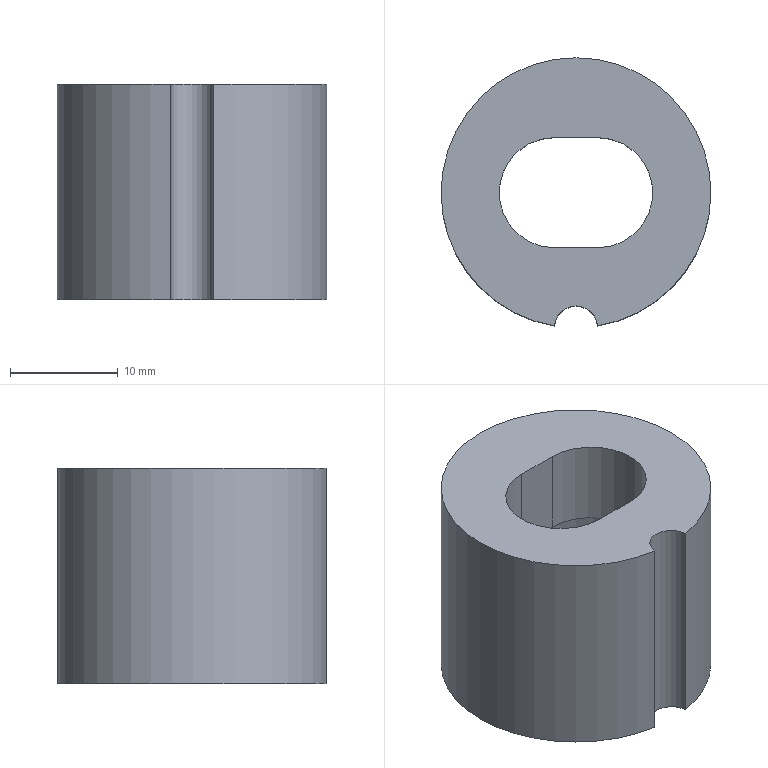Part | NX | features solid 2 | 1 solid | 10 faces | box 25 x 24.84 x 20 mm | volume 6116 mm3 | plane 5 | cylinder 5 | commonest cylinder face diameters 10.22 x2 4 x1 16.6 x1 25 x1
STEP:
#1=CARTESIAN_POINT('',(299.802,7.404,-5.344));
#2=VERTEX_POINT('',#1);
#3=CARTESIAN_POINT('',(303.789,7.404,-5.344));
#4=VERTEX_POINT('',#3);
#5=CARTESIAN_POINT('',(301.795,7.244,-5.344));
#6=DIRECTION('',(0.,0.,-1.));
#7=DIRECTION('',(0.,1.,0.));
#8=AXIS2_PLACEMENT_3D('',#5,#6,#7);
#9=CIRCLE('',#8,2.);
#10=EDGE_CURVE('',#2,#4,#9,.T.);
#11=ORIENTED_EDGE('',*,*,#10,.T.);
#12=CARTESIAN_POINT('',(301.795,19.744,-5.344));
#13=DIRECTION('',(0.,0.,-1.));
#14=DIRECTION('',(0.,1.,0.));
#15=AXIS2_PLACEMENT_3D('',#12,#13,#14);
#16=CIRCLE('',#15,12.5);
#17=EDGE_CURVE('',#2,#4,#16,.T.);
#18=ORIENTED_EDGE('',*,*,#17,.F.);
#19=EDGE_LOOP('',(#11,#18));
#20=FACE_BOUND('',#19,.T.);
#21=CARTESIAN_POINT('',(303.795,24.854,-5.344));
#22=VERTEX_POINT('',#21);
#23=CARTESIAN_POINT('',(303.795,14.634,-5.344));
#24=VERTEX_POINT('',#23);
#25=CARTESIAN_POINT('',(303.795,19.744,-5.344));
#26=DIRECTION('',(0.,0.,-1.));
#27=DIRECTION('',(0.,1.,0.));
#28=AXIS2_PLACEMENT_3D('',#25,#26,#27);
#29=CIRCLE('',#28,5.11);
#30=EDGE_CURVE('',#22,#24,#29,.T.);
#31=ORIENTED_EDGE('',*,*,#30,.T.);
#32=CARTESIAN_POINT('',(299.795,14.634,-5.344));
#33=VERTEX_POINT('',#32);
#34=CARTESIAN_POINT('',(301.795,14.634,-5.344));
#35=DIRECTION('',(-1.,0.,0.));
#36=VECTOR('',#35,1000.);
#37=LINE('',#34,#36);
#38=EDGE_CURVE('',#24,#33,#37,.T.);
#39=ORIENTED_EDGE('',*,*,#38,.T.);
#40=CARTESIAN_POINT('',(299.795,24.854,-5.344));
#41=VERTEX_POINT('',#40);
#42=CARTESIAN_POINT('',(299.795,19.744,-5.344));
#43=DIRECTION('',(0.,0.,-1.));
#44=DIRECTION('',(0.,1.,0.));
#45=AXIS2_PLACEMENT_3D('',#42,#43,#44);
#46=CIRCLE('',#45,5.11);
#47=EDGE_CURVE('',#33,#41,#46,.T.);
#48=ORIENTED_EDGE('',*,*,#47,.T.);
#49=CARTESIAN_POINT('',(301.795,24.854,-5.344));
#50=DIRECTION('',(1.,0.,0.));
#51=VECTOR('',#50,1000.);
#52=LINE('',#49,#51);
#53=EDGE_CURVE('',#41,#22,#52,.T.);
#54=ORIENTED_EDGE('',*,*,#53,.T.);
#55=EDGE_LOOP('',(#31,#39,#48,#54));
#56=FACE_BOUND('',#55,.T.);
#57=CARTESIAN_POINT('',(301.795,19.744,-5.344));
#58=DIRECTION('',(0.,0.,1.));
#59=DIRECTION('',(0.,-1.,0.));
#60=AXIS2_PLACEMENT_3D('',#57,#58,#59);
#61=PLANE('',#60);
#62=ADVANCED_FACE('',(#20,#56),#61,.T.);
#63=CARTESIAN_POINT('',(303.789,7.404,-25.344));
#64=VERTEX_POINT('',#63);
#65=CARTESIAN_POINT('',(299.802,7.404,-25.344));
#66=VERTEX_POINT('',#65);
#67=CARTESIAN_POINT('',(301.795,7.244,-25.344));
#68=DIRECTION('',(0.,0.,1.));
#69=DIRECTION('',(0.,-1.,0.));
#70=AXIS2_PLACEMENT_3D('',#67,#68,#69);
#71=CIRCLE('',#70,2.);
#72=EDGE_CURVE('',#64,#66,#71,.T.);
#73=ORIENTED_EDGE('',*,*,#72,.T.);
#74=CARTESIAN_POINT('',(301.795,19.744,-25.344));
#75=DIRECTION('',(0.,0.,1.));
#76=DIRECTION('',(0.,-1.,0.));
#77=AXIS2_PLACEMENT_3D('',#74,#75,#76);
#78=CIRCLE('',#77,12.5);
#79=EDGE_CURVE('',#64,#66,#78,.T.);
#80=ORIENTED_EDGE('',*,*,#79,.F.);
#81=EDGE_LOOP('',(#73,#80));
#82=FACE_BOUND('',#81,.T.);
#83=CARTESIAN_POINT('',(301.795,11.444,-25.344));
#84=VERTEX_POINT('',#83);
#85=CARTESIAN_POINT('',(301.795,19.744,-25.344));
#86=DIRECTION('',(0.,0.,1.));
#87=DIRECTION('',(0.,-1.,0.));
#88=AXIS2_PLACEMENT_3D('',#85,#86,#87);
#89=CIRCLE('',#88,8.3);
#90=EDGE_CURVE('',#84,#84,#89,.T.);
#91=ORIENTED_EDGE('',*,*,#90,.T.);
#92=EDGE_LOOP('',(#91));
#93=FACE_BOUND('',#92,.T.);
#94=CARTESIAN_POINT('',(301.795,19.744,-25.344));
#95=DIRECTION('',(0.,0.,-1.));
#96=DIRECTION('',(0.,1.,0.));
#97=AXIS2_PLACEMENT_3D('',#94,#95,#96);
#98=PLANE('',#97);
#99=ADVANCED_FACE('',(#82,#93),#98,.T.);
#100=CARTESIAN_POINT('',(303.789,7.404,-15.344));
#101=DIRECTION('',(0.,0.,1.));
#102=VECTOR('',#101,1000.);
#103=LINE('',#100,#102);
#104=EDGE_CURVE('',#64,#4,#103,.T.);
#105=ORIENTED_EDGE('',*,*,#104,.F.);
#106=ORIENTED_EDGE('',*,*,#79,.T.);
#107=CARTESIAN_POINT('',(299.802,7.404,-15.344));
#108=DIRECTION('',(0.,0.,1.));
#109=VECTOR('',#108,1000.);
#110=LINE('',#107,#109);
#111=EDGE_CURVE('',#2,#66,#110,.F.);
#112=ORIENTED_EDGE('',*,*,#111,.F.);
#113=ORIENTED_EDGE('',*,*,#17,.T.);
#114=EDGE_LOOP('',(#105,#106,#112,#113));
#115=FACE_BOUND('',#114,.T.);
#116=CARTESIAN_POINT('',(301.795,19.744,-25.344));
#117=DIRECTION('',(0.,0.,1.));
#118=DIRECTION('',(0.,-1.,0.));
#119=AXIS2_PLACEMENT_3D('',#116,#117,#118);
#120=CYLINDRICAL_SURFACE('',#119,12.5);
#121=ADVANCED_FACE('',(#115),#120,.T.);
#122=CARTESIAN_POINT('',(299.795,14.634,-13.344));
#123=VERTEX_POINT('',#122);
#124=CARTESIAN_POINT('',(303.795,14.634,-13.344));
#125=VERTEX_POINT('',#124);
#126=CARTESIAN_POINT('',(301.795,14.634,-13.344));
#127=DIRECTION('',(1.,0.,0.));
#128=VECTOR('',#127,1000.);
#129=LINE('',#126,#128);
#130=EDGE_CURVE('',#123,#125,#129,.T.);
#131=ORIENTED_EDGE('',*,*,#130,.T.);
#132=CARTESIAN_POINT('',(303.795,24.854,-13.344));
#133=VERTEX_POINT('',#132);
#134=CARTESIAN_POINT('',(303.795,19.744,-13.344));
#135=DIRECTION('',(0.,0.,1.));
#136=DIRECTION('',(0.,-1.,0.));
#137=AXIS2_PLACEMENT_3D('',#134,#135,#136);
#138=CIRCLE('',#137,5.11);
#139=EDGE_CURVE('',#125,#133,#138,.T.);
#140=ORIENTED_EDGE('',*,*,#139,.T.);
#141=CARTESIAN_POINT('',(299.795,24.854,-13.344));
#142=VERTEX_POINT('',#141);
#143=CARTESIAN_POINT('',(301.795,24.854,-13.344));
#144=DIRECTION('',(-1.,0.,0.));
#145=VECTOR('',#144,1000.);
#146=LINE('',#143,#145);
#147=EDGE_CURVE('',#133,#142,#146,.T.);
#148=ORIENTED_EDGE('',*,*,#147,.T.);
#149=CARTESIAN_POINT('',(299.795,19.744,-13.344));
#150=DIRECTION('',(0.,0.,1.));
#151=DIRECTION('',(0.,-1.,0.));
#152=AXIS2_PLACEMENT_3D('',#149,#150,#151);
#153=CIRCLE('',#152,5.11);
#154=EDGE_CURVE('',#142,#123,#153,.T.);
#155=ORIENTED_EDGE('',*,*,#154,.T.);
#156=EDGE_LOOP('',(#131,#140,#148,#155));
#157=FACE_BOUND('',#156,.T.);
#158=CARTESIAN_POINT('',(301.795,28.044,-13.344));
#159=VERTEX_POINT('',#158);
#160=CARTESIAN_POINT('',(301.795,19.744,-13.344));
#161=DIRECTION('',(0.,0.,-1.));
#162=DIRECTION('',(0.,1.,0.));
#163=AXIS2_PLACEMENT_3D('',#160,#161,#162);
#164=CIRCLE('',#163,8.3);
#165=EDGE_CURVE('',#159,#159,#164,.T.);
#166=ORIENTED_EDGE('',*,*,#165,.T.);
#167=EDGE_LOOP('',(#166));
#168=FACE_BOUND('',#167,.T.);
#169=CARTESIAN_POINT('',(301.795,19.744,-13.344));
#170=DIRECTION('',(0.,0.,1.));
#171=DIRECTION('',(0.,-1.,0.));
#172=AXIS2_PLACEMENT_3D('',#169,#170,#171);
#173=PLANE('',#172);
#174=ADVANCED_FACE('',(#157,#168),#173,.F.);
#175=ORIENTED_EDGE('',*,*,#165,.F.);
#176=EDGE_LOOP('',(#175));
#177=FACE_BOUND('',#176,.T.);
#178=ORIENTED_EDGE('',*,*,#90,.F.);
#179=EDGE_LOOP('',(#178));
#180=FACE_BOUND('',#179,.T.);
#181=CARTESIAN_POINT('',(301.795,19.744,-25.344));
#182=DIRECTION('',(0.,0.,1.));
#183=DIRECTION('',(0.,-1.,0.));
#184=AXIS2_PLACEMENT_3D('',#181,#182,#183);
#185=CYLINDRICAL_SURFACE('',#184,8.3);
#186=ADVANCED_FACE('',(#177,#180),#185,.F.);
#187=CARTESIAN_POINT('',(299.795,24.854,-13.344));
#188=DIRECTION('',(0.,0.,1.));
#189=VECTOR('',#188,1000.);
#190=LINE('',#187,#189);
#191=EDGE_CURVE('',#142,#41,#190,.T.);
#192=ORIENTED_EDGE('',*,*,#191,.F.);
#193=ORIENTED_EDGE('',*,*,#147,.F.);
#194=CARTESIAN_POINT('',(303.795,24.854,-13.344));
#195=DIRECTION('',(0.,0.,1.));
#196=VECTOR('',#195,1000.);
#197=LINE('',#194,#196);
#198=EDGE_CURVE('',#133,#22,#197,.T.);
#199=ORIENTED_EDGE('',*,*,#198,.T.);
#200=ORIENTED_EDGE('',*,*,#53,.F.);
#201=EDGE_LOOP('',(#192,#193,#199,#200));
#202=FACE_BOUND('',#201,.T.);
#203=CARTESIAN_POINT('',(301.795,24.854,-13.344));
#204=DIRECTION('',(0.,1.,0.));
#205=DIRECTION('',(0.,0.,1.));
#206=AXIS2_PLACEMENT_3D('',#203,#204,#205);
#207=PLANE('',#206);
#208=ADVANCED_FACE('',(#202),#207,.F.);
#209=ORIENTED_EDGE('',*,*,#130,.F.);
#210=CARTESIAN_POINT('',(299.795,14.634,-13.344));
#211=DIRECTION('',(0.,0.,1.));
#212=VECTOR('',#211,1000.);
#213=LINE('',#210,#212);
#214=EDGE_CURVE('',#123,#33,#213,.T.);
#215=ORIENTED_EDGE('',*,*,#214,.T.);
#216=ORIENTED_EDGE('',*,*,#38,.F.);
#217=CARTESIAN_POINT('',(303.795,14.634,-13.344));
#218=DIRECTION('',(0.,0.,1.));
#219=VECTOR('',#218,1000.);
#220=LINE('',#217,#219);
#221=EDGE_CURVE('',#125,#24,#220,.T.);
#222=ORIENTED_EDGE('',*,*,#221,.F.);
#223=EDGE_LOOP('',(#209,#215,#216,#222));
#224=FACE_BOUND('',#223,.T.);
#225=CARTESIAN_POINT('',(301.795,14.634,-13.344));
#226=DIRECTION('',(0.,-1.,0.));
#227=DIRECTION('',(0.,0.,-1.));
#228=AXIS2_PLACEMENT_3D('',#225,#226,#227);
#229=PLANE('',#228);
#230=ADVANCED_FACE('',(#224),#229,.F.);
#231=ORIENTED_EDGE('',*,*,#191,.T.);
#232=ORIENTED_EDGE('',*,*,#47,.F.);
#233=ORIENTED_EDGE('',*,*,#214,.F.);
#234=ORIENTED_EDGE('',*,*,#154,.F.);
#235=EDGE_LOOP('',(#231,#232,#233,#234));
#236=FACE_BOUND('',#235,.T.);
#237=CARTESIAN_POINT('',(299.795,19.744,-13.344));
#238=DIRECTION('',(0.,0.,1.));
#239=DIRECTION('',(0.,-1.,0.));
#240=AXIS2_PLACEMENT_3D('',#237,#238,#239);
#241=CYLINDRICAL_SURFACE('',#240,5.11);
#242=ADVANCED_FACE('',(#236),#241,.F.);
#243=ORIENTED_EDGE('',*,*,#139,.F.);
#244=ORIENTED_EDGE('',*,*,#221,.T.);
#245=ORIENTED_EDGE('',*,*,#30,.F.);
#246=ORIENTED_EDGE('',*,*,#198,.F.);
#247=EDGE_LOOP('',(#243,#244,#245,#246));
#248=FACE_BOUND('',#247,.T.);
#249=CARTESIAN_POINT('',(303.795,19.744,-13.344));
#250=DIRECTION('',(0.,0.,1.));
#251=DIRECTION('',(0.,-1.,0.));
#252=AXIS2_PLACEMENT_3D('',#249,#250,#251);
#253=CYLINDRICAL_SURFACE('',#252,5.11);
#254=ADVANCED_FACE('',(#248),#253,.F.);
#255=ORIENTED_EDGE('',*,*,#104,.T.);
#256=ORIENTED_EDGE('',*,*,#10,.F.);
#257=ORIENTED_EDGE('',*,*,#111,.T.);
#258=ORIENTED_EDGE('',*,*,#72,.F.);
#259=EDGE_LOOP('',(#255,#256,#257,#258));
#260=FACE_BOUND('',#259,.T.);
#261=CARTESIAN_POINT('',(301.795,7.244,-25.344));
#262=DIRECTION('',(0.,0.,1.));
#263=DIRECTION('',(0.,-1.,0.));
#264=AXIS2_PLACEMENT_3D('',#261,#262,#263);
#265=CYLINDRICAL_SURFACE('',#264,2.);
#266=ADVANCED_FACE('',(#260),#265,.F.);
#267=CLOSED_SHELL('',(#62,#99,#121,#174,#186,#208,#230,#242,#254,#266));
#268=MANIFOLD_SOLID_BREP('',#267);
#269=(LENGTH_UNIT()NAMED_UNIT(*)SI_UNIT(.MILLI.,.METRE.));
#270=UNCERTAINTY_MEASURE_WITH_UNIT(LENGTH_MEASURE(0.00001),#269,'','');
#271=(NAMED_UNIT(*)PLANE_ANGLE_UNIT()SI_UNIT($,.RADIAN.));
#272=(NAMED_UNIT(*)SI_UNIT($,.STERADIAN.)SOLID_ANGLE_UNIT());
#273=(GEOMETRIC_REPRESENTATION_CONTEXT(3)GLOBAL_UNCERTAINTY_ASSIGNED_CONTEXT((#270))GLOBAL_UNIT_ASSIGNED_CONTEXT((#269,#271,#272))REPRESENTATION_CONTEXT('',''));
#274=ADVANCED_BREP_SHAPE_REPRESENTATION('',(#268),#273);